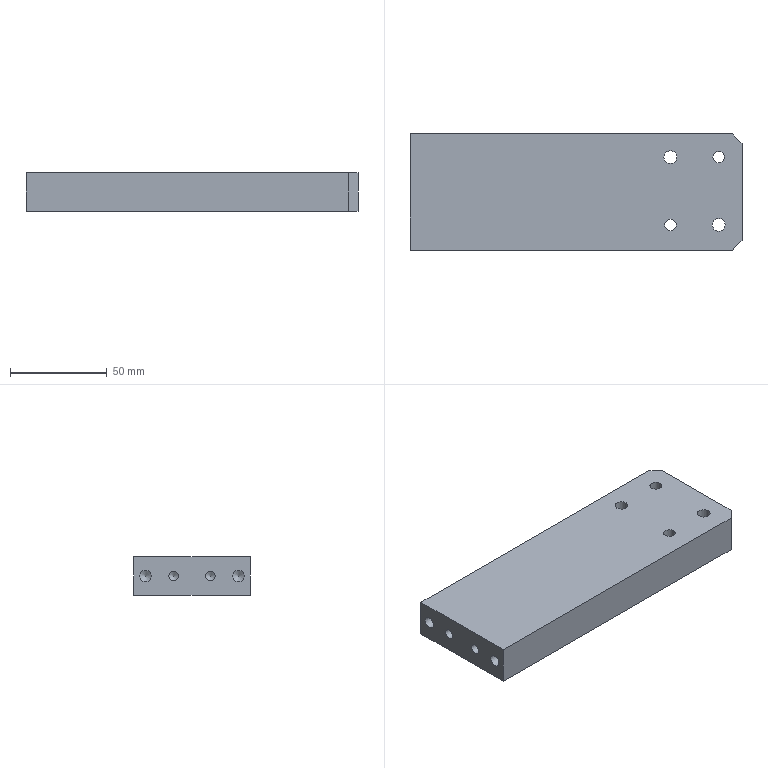Part | NX | features BREP 1 | 1 solid | 24 faces | box 171.5 x 60 x 20 mm | volume 200701 mm3 | plane 10 | cylinder 10 | cone 4 | commonest cylinder face diameters 6 x4 5 x2 6.6 x2 11 x2
STEP:
#1=CARTESIAN_POINT('',(-85.75,-30.,20.));
#2=VERTEX_POINT('',#1);
#3=CARTESIAN_POINT('',(80.75,-30.,20.));
#4=VERTEX_POINT('',#3);
#5=CARTESIAN_POINT('',(0.,-30.,20.));
#6=DIRECTION('',(1.,0.,0.));
#7=VECTOR('',#6,1000.);
#8=LINE('',#5,#7);
#9=EDGE_CURVE('',#2,#4,#8,.T.);
#10=ORIENTED_EDGE('',*,*,#9,.T.);
#11=CARTESIAN_POINT('',(85.75,-25.,20.));
#12=VERTEX_POINT('',#11);
#13=CARTESIAN_POINT('',(80.75,-30.,20.));
#14=DIRECTION('',(0.7071,0.7071,0.));
#15=VECTOR('',#14,1000.);
#16=LINE('',#13,#15);
#17=EDGE_CURVE('',#4,#12,#16,.T.);
#18=ORIENTED_EDGE('',*,*,#17,.T.);
#19=CARTESIAN_POINT('',(85.75,25.,20.));
#20=VERTEX_POINT('',#19);
#21=CARTESIAN_POINT('',(85.75,0.,20.));
#22=DIRECTION('',(0.,1.,0.));
#23=VECTOR('',#22,1000.);
#24=LINE('',#21,#23);
#25=EDGE_CURVE('',#12,#20,#24,.T.);
#26=ORIENTED_EDGE('',*,*,#25,.T.);
#27=CARTESIAN_POINT('',(80.75,30.,20.));
#28=VERTEX_POINT('',#27);
#29=CARTESIAN_POINT('',(85.75,25.,20.));
#30=DIRECTION('',(-0.7071,0.7071,0.));
#31=VECTOR('',#30,1000.);
#32=LINE('',#29,#31);
#33=EDGE_CURVE('',#20,#28,#32,.T.);
#34=ORIENTED_EDGE('',*,*,#33,.T.);
#35=CARTESIAN_POINT('',(-85.75,30.,20.));
#36=VERTEX_POINT('',#35);
#37=CARTESIAN_POINT('',(0.,30.,20.));
#38=DIRECTION('',(-1.,0.,0.));
#39=VECTOR('',#38,1000.);
#40=LINE('',#37,#39);
#41=EDGE_CURVE('',#28,#36,#40,.T.);
#42=ORIENTED_EDGE('',*,*,#41,.T.);
#43=CARTESIAN_POINT('',(-85.75,0.,20.));
#44=DIRECTION('',(0.,-1.,0.));
#45=VECTOR('',#44,1000.);
#46=LINE('',#43,#45);
#47=EDGE_CURVE('',#36,#2,#46,.T.);
#48=ORIENTED_EDGE('',*,*,#47,.T.);
#49=EDGE_LOOP('',(#10,#18,#26,#34,#42,#48));
#50=FACE_BOUND('',#49,.T.);
#51=CARTESIAN_POINT('',(51.75,-17.,20.));
#52=VERTEX_POINT('',#51);
#53=CARTESIAN_POINT('',(48.75,-17.,20.));
#54=DIRECTION('',(0.,0.,-1.));
#55=DIRECTION('',(1.,0.,0.));
#56=AXIS2_PLACEMENT_3D('',#53,#54,#55);
#57=CIRCLE('',#56,3.);
#58=EDGE_CURVE('',#52,#52,#57,.T.);
#59=ORIENTED_EDGE('',*,*,#58,.T.);
#60=EDGE_LOOP('',(#59));
#61=FACE_BOUND('',#60,.T.);
#62=CARTESIAN_POINT('',(76.75,18.,20.));
#63=VERTEX_POINT('',#62);
#64=CARTESIAN_POINT('',(73.75,18.,20.));
#65=DIRECTION('',(0.,0.,-1.));
#66=DIRECTION('',(1.,0.,0.));
#67=AXIS2_PLACEMENT_3D('',#64,#65,#66);
#68=CIRCLE('',#67,3.);
#69=EDGE_CURVE('',#63,#63,#68,.T.);
#70=ORIENTED_EDGE('',*,*,#69,.T.);
#71=EDGE_LOOP('',(#70));
#72=FACE_BOUND('',#71,.T.);
#73=CARTESIAN_POINT('',(45.45,18.,20.));
#74=VERTEX_POINT('',#73);
#75=CARTESIAN_POINT('',(48.75,18.,20.));
#76=DIRECTION('',(0.,0.,-1.));
#77=DIRECTION('',(-1.,0.,0.));
#78=AXIS2_PLACEMENT_3D('',#75,#76,#77);
#79=CIRCLE('',#78,3.3);
#80=EDGE_CURVE('',#74,#74,#79,.T.);
#81=ORIENTED_EDGE('',*,*,#80,.T.);
#82=EDGE_LOOP('',(#81));
#83=FACE_BOUND('',#82,.T.);
#84=CARTESIAN_POINT('',(70.45,-17.,20.));
#85=VERTEX_POINT('',#84);
#86=CARTESIAN_POINT('',(73.75,-17.,20.));
#87=DIRECTION('',(0.,0.,-1.));
#88=DIRECTION('',(-1.,0.,0.));
#89=AXIS2_PLACEMENT_3D('',#86,#87,#88);
#90=CIRCLE('',#89,3.3);
#91=EDGE_CURVE('',#85,#85,#90,.T.);
#92=ORIENTED_EDGE('',*,*,#91,.T.);
#93=EDGE_LOOP('',(#92));
#94=FACE_BOUND('',#93,.T.);
#95=CARTESIAN_POINT('',(0.,0.,20.));
#96=DIRECTION('',(0.,0.,1.));
#97=DIRECTION('',(-1.,0.,0.));
#98=AXIS2_PLACEMENT_3D('',#95,#96,#97);
#99=PLANE('',#98);
#100=ADVANCED_FACE('',(#50,#61,#72,#83,#94),#99,.T.);
#101=CARTESIAN_POINT('',(80.75,-30.,0.));
#102=VERTEX_POINT('',#101);
#103=CARTESIAN_POINT('',(80.75,-30.,20.));
#104=DIRECTION('',(0.,0.,1.));
#105=VECTOR('',#104,1000.);
#106=LINE('',#103,#105);
#107=EDGE_CURVE('',#102,#4,#106,.T.);
#108=ORIENTED_EDGE('',*,*,#107,.F.);
#109=CARTESIAN_POINT('',(85.75,-25.,0.));
#110=VERTEX_POINT('',#109);
#111=CARTESIAN_POINT('',(85.75,-25.,0.));
#112=DIRECTION('',(-0.7071,-0.7071,0.));
#113=VECTOR('',#112,1000.);
#114=LINE('',#111,#113);
#115=EDGE_CURVE('',#110,#102,#114,.T.);
#116=ORIENTED_EDGE('',*,*,#115,.F.);
#117=CARTESIAN_POINT('',(85.75,-25.,20.));
#118=DIRECTION('',(0.,0.,-1.));
#119=VECTOR('',#118,1000.);
#120=LINE('',#117,#119);
#121=EDGE_CURVE('',#12,#110,#120,.T.);
#122=ORIENTED_EDGE('',*,*,#121,.F.);
#123=ORIENTED_EDGE('',*,*,#17,.F.);
#124=EDGE_LOOP('',(#108,#116,#122,#123));
#125=FACE_BOUND('',#124,.T.);
#126=CARTESIAN_POINT('',(85.75,-25.,20.));
#127=DIRECTION('',(-0.7071,0.7071,0.));
#128=DIRECTION('',(0.7071,0.7071,0.));
#129=AXIS2_PLACEMENT_3D('',#126,#127,#128);
#130=PLANE('',#129);
#131=ADVANCED_FACE('',(#125),#130,.F.);
#132=ORIENTED_EDGE('',*,*,#107,.T.);
#133=ORIENTED_EDGE('',*,*,#9,.F.);
#134=CARTESIAN_POINT('',(-85.75,-30.,0.));
#135=VERTEX_POINT('',#134);
#136=CARTESIAN_POINT('',(-85.75,-30.,20.));
#137=DIRECTION('',(0.,0.,1.));
#138=VECTOR('',#137,1000.);
#139=LINE('',#136,#138);
#140=EDGE_CURVE('',#135,#2,#139,.T.);
#141=ORIENTED_EDGE('',*,*,#140,.F.);
#142=CARTESIAN_POINT('',(-85.75,-30.,0.));
#143=DIRECTION('',(-1.,0.,0.));
#144=VECTOR('',#143,1000.);
#145=LINE('',#142,#144);
#146=EDGE_CURVE('',#102,#135,#145,.T.);
#147=ORIENTED_EDGE('',*,*,#146,.F.);
#148=EDGE_LOOP('',(#132,#133,#141,#147));
#149=FACE_BOUND('',#148,.T.);
#150=CARTESIAN_POINT('',(-85.75,-30.,20.));
#151=DIRECTION('',(0.,1.,0.));
#152=DIRECTION('',(0.,0.,-1.));
#153=AXIS2_PLACEMENT_3D('',#150,#151,#152);
#154=PLANE('',#153);
#155=ADVANCED_FACE('',(#149),#154,.F.);
#156=ORIENTED_EDGE('',*,*,#140,.T.);
#157=ORIENTED_EDGE('',*,*,#47,.F.);
#158=CARTESIAN_POINT('',(-85.75,30.,0.));
#159=VERTEX_POINT('',#158);
#160=CARTESIAN_POINT('',(-85.75,30.,20.));
#161=DIRECTION('',(0.,0.,1.));
#162=VECTOR('',#161,1000.);
#163=LINE('',#160,#162);
#164=EDGE_CURVE('',#159,#36,#163,.T.);
#165=ORIENTED_EDGE('',*,*,#164,.F.);
#166=CARTESIAN_POINT('',(-85.75,30.,0.));
#167=DIRECTION('',(0.,1.,0.));
#168=VECTOR('',#167,1000.);
#169=LINE('',#166,#168);
#170=EDGE_CURVE('',#135,#159,#169,.T.);
#171=ORIENTED_EDGE('',*,*,#170,.F.);
#172=EDGE_LOOP('',(#156,#157,#165,#171));
#173=FACE_BOUND('',#172,.T.);
#174=CARTESIAN_POINT('',(-85.75,-24.,13.));
#175=VERTEX_POINT('',#174);
#176=CARTESIAN_POINT('',(-85.75,-24.,10.));
#177=DIRECTION('',(-1.,0.,0.));
#178=DIRECTION('',(0.,0.,1.));
#179=AXIS2_PLACEMENT_3D('',#176,#177,#178);
#180=CIRCLE('',#179,3.);
#181=EDGE_CURVE('',#175,#175,#180,.T.);
#182=ORIENTED_EDGE('',*,*,#181,.F.);
#183=EDGE_LOOP('',(#182));
#184=FACE_BOUND('',#183,.T.);
#185=CARTESIAN_POINT('',(-85.75,24.,13.));
#186=VERTEX_POINT('',#185);
#187=CARTESIAN_POINT('',(-85.75,24.,10.));
#188=DIRECTION('',(-1.,0.,0.));
#189=DIRECTION('',(0.,0.,1.));
#190=AXIS2_PLACEMENT_3D('',#187,#188,#189);
#191=CIRCLE('',#190,3.);
#192=EDGE_CURVE('',#186,#186,#191,.T.);
#193=ORIENTED_EDGE('',*,*,#192,.F.);
#194=EDGE_LOOP('',(#193));
#195=FACE_BOUND('',#194,.T.);
#196=CARTESIAN_POINT('',(-85.75,9.5,12.5));
#197=VERTEX_POINT('',#196);
#198=CARTESIAN_POINT('',(-85.75,9.5,10.));
#199=DIRECTION('',(-1.,0.,0.));
#200=DIRECTION('',(0.,0.,1.));
#201=AXIS2_PLACEMENT_3D('',#198,#199,#200);
#202=CIRCLE('',#201,2.5);
#203=EDGE_CURVE('',#197,#197,#202,.T.);
#204=ORIENTED_EDGE('',*,*,#203,.F.);
#205=EDGE_LOOP('',(#204));
#206=FACE_BOUND('',#205,.T.);
#207=CARTESIAN_POINT('',(-85.75,-9.5,12.5));
#208=VERTEX_POINT('',#207);
#209=CARTESIAN_POINT('',(-85.75,-9.5,10.));
#210=DIRECTION('',(-1.,0.,0.));
#211=DIRECTION('',(0.,0.,1.));
#212=AXIS2_PLACEMENT_3D('',#209,#210,#211);
#213=CIRCLE('',#212,2.5);
#214=EDGE_CURVE('',#208,#208,#213,.T.);
#215=ORIENTED_EDGE('',*,*,#214,.F.);
#216=EDGE_LOOP('',(#215));
#217=FACE_BOUND('',#216,.T.);
#218=CARTESIAN_POINT('',(-85.75,30.,20.));
#219=DIRECTION('',(1.,0.,0.));
#220=DIRECTION('',(0.,-1.,0.));
#221=AXIS2_PLACEMENT_3D('',#218,#219,#220);
#222=PLANE('',#221);
#223=ADVANCED_FACE('',(#173,#184,#195,#206,#217),#222,.F.);
#224=CARTESIAN_POINT('',(80.75,30.,0.));
#225=VERTEX_POINT('',#224);
#226=CARTESIAN_POINT('',(80.75,30.,20.));
#227=DIRECTION('',(0.,0.,1.));
#228=VECTOR('',#227,1000.);
#229=LINE('',#226,#228);
#230=EDGE_CURVE('',#225,#28,#229,.T.);
#231=ORIENTED_EDGE('',*,*,#230,.F.);
#232=CARTESIAN_POINT('',(-85.75,30.,0.));
#233=DIRECTION('',(1.,0.,0.));
#234=VECTOR('',#233,1000.);
#235=LINE('',#232,#234);
#236=EDGE_CURVE('',#159,#225,#235,.T.);
#237=ORIENTED_EDGE('',*,*,#236,.F.);
#238=ORIENTED_EDGE('',*,*,#164,.T.);
#239=ORIENTED_EDGE('',*,*,#41,.F.);
#240=EDGE_LOOP('',(#231,#237,#238,#239));
#241=FACE_BOUND('',#240,.T.);
#242=CARTESIAN_POINT('',(-85.75,30.,20.));
#243=DIRECTION('',(0.,-1.,0.));
#244=DIRECTION('',(0.,0.,1.));
#245=AXIS2_PLACEMENT_3D('',#242,#243,#244);
#246=PLANE('',#245);
#247=ADVANCED_FACE('',(#241),#246,.F.);
#248=CARTESIAN_POINT('',(85.75,25.,0.));
#249=VERTEX_POINT('',#248);
#250=CARTESIAN_POINT('',(85.75,25.,20.));
#251=DIRECTION('',(0.,0.,1.));
#252=VECTOR('',#251,1000.);
#253=LINE('',#250,#252);
#254=EDGE_CURVE('',#249,#20,#253,.T.);
#255=ORIENTED_EDGE('',*,*,#254,.F.);
#256=CARTESIAN_POINT('',(80.75,30.,0.));
#257=DIRECTION('',(0.7071,-0.7071,0.));
#258=VECTOR('',#257,1000.);
#259=LINE('',#256,#258);
#260=EDGE_CURVE('',#225,#249,#259,.T.);
#261=ORIENTED_EDGE('',*,*,#260,.F.);
#262=ORIENTED_EDGE('',*,*,#230,.T.);
#263=ORIENTED_EDGE('',*,*,#33,.F.);
#264=EDGE_LOOP('',(#255,#261,#262,#263));
#265=FACE_BOUND('',#264,.T.);
#266=CARTESIAN_POINT('',(80.75,30.,20.));
#267=DIRECTION('',(-0.7071,-0.7071,0.));
#268=DIRECTION('',(-0.7071,0.7071,0.));
#269=AXIS2_PLACEMENT_3D('',#266,#267,#268);
#270=PLANE('',#269);
#271=ADVANCED_FACE('',(#265),#270,.F.);
#272=ORIENTED_EDGE('',*,*,#254,.T.);
#273=ORIENTED_EDGE('',*,*,#25,.F.);
#274=ORIENTED_EDGE('',*,*,#121,.T.);
#275=CARTESIAN_POINT('',(85.75,30.,0.));
#276=DIRECTION('',(0.,-1.,0.));
#277=VECTOR('',#276,1000.);
#278=LINE('',#275,#277);
#279=EDGE_CURVE('',#249,#110,#278,.T.);
#280=ORIENTED_EDGE('',*,*,#279,.F.);
#281=EDGE_LOOP('',(#272,#273,#274,#280));
#282=FACE_BOUND('',#281,.T.);
#283=CARTESIAN_POINT('',(85.75,30.,20.));
#284=DIRECTION('',(-1.,0.,0.));
#285=DIRECTION('',(0.,1.,0.));
#286=AXIS2_PLACEMENT_3D('',#283,#284,#285);
#287=PLANE('',#286);
#288=ADVANCED_FACE('',(#282),#287,.F.);
#289=ORIENTED_EDGE('',*,*,#58,.F.);
#290=EDGE_LOOP('',(#289));
#291=FACE_BOUND('',#290,.T.);
#292=CARTESIAN_POINT('',(51.75,-17.,0.));
#293=VERTEX_POINT('',#292);
#294=CARTESIAN_POINT('',(48.75,-17.,0.));
#295=DIRECTION('',(0.,0.,1.));
#296=DIRECTION('',(1.,0.,0.));
#297=AXIS2_PLACEMENT_3D('',#294,#295,#296);
#298=CIRCLE('',#297,3.);
#299=EDGE_CURVE('',#293,#293,#298,.T.);
#300=ORIENTED_EDGE('',*,*,#299,.F.);
#301=EDGE_LOOP('',(#300));
#302=FACE_BOUND('',#301,.T.);
#303=CARTESIAN_POINT('',(48.75,-17.,20.));
#304=DIRECTION('',(0.,0.,1.));
#305=DIRECTION('',(-1.,0.,0.));
#306=AXIS2_PLACEMENT_3D('',#303,#304,#305);
#307=CYLINDRICAL_SURFACE('',#306,3.);
#308=ADVANCED_FACE('',(#291,#302),#307,.F.);
#309=ORIENTED_EDGE('',*,*,#69,.F.);
#310=EDGE_LOOP('',(#309));
#311=FACE_BOUND('',#310,.T.);
#312=CARTESIAN_POINT('',(76.75,18.,0.));
#313=VERTEX_POINT('',#312);
#314=CARTESIAN_POINT('',(73.75,18.,0.));
#315=DIRECTION('',(0.,0.,1.));
#316=DIRECTION('',(1.,0.,0.));
#317=AXIS2_PLACEMENT_3D('',#314,#315,#316);
#318=CIRCLE('',#317,3.);
#319=EDGE_CURVE('',#313,#313,#318,.T.);
#320=ORIENTED_EDGE('',*,*,#319,.F.);
#321=EDGE_LOOP('',(#320));
#322=FACE_BOUND('',#321,.T.);
#323=CARTESIAN_POINT('',(73.75,18.,20.));
#324=DIRECTION('',(0.,0.,1.));
#325=DIRECTION('',(-1.,0.,0.));
#326=AXIS2_PLACEMENT_3D('',#323,#324,#325);
#327=CYLINDRICAL_SURFACE('',#326,3.);
#328=ADVANCED_FACE('',(#311,#322),#327,.F.);
#329=CARTESIAN_POINT('',(45.45,18.,6.4));
#330=VERTEX_POINT('',#329);
#331=CARTESIAN_POINT('',(48.75,18.,6.4));
#332=DIRECTION('',(0.,0.,1.));
#333=DIRECTION('',(-1.,0.,0.));
#334=AXIS2_PLACEMENT_3D('',#331,#332,#333);
#335=CIRCLE('',#334,3.3);
#336=EDGE_CURVE('',#330,#330,#335,.T.);
#337=ORIENTED_EDGE('',*,*,#336,.F.);
#338=EDGE_LOOP('',(#337));
#339=FACE_BOUND('',#338,.T.);
#340=ORIENTED_EDGE('',*,*,#80,.F.);
#341=EDGE_LOOP('',(#340));
#342=FACE_BOUND('',#341,.T.);
#343=CARTESIAN_POINT('',(48.75,18.,0.));
#344=DIRECTION('',(0.,0.,-1.));
#345=DIRECTION('',(1.,0.,0.));
#346=AXIS2_PLACEMENT_3D('',#343,#344,#345);
#347=CYLINDRICAL_SURFACE('',#346,3.3);
#348=ADVANCED_FACE('',(#339,#342),#347,.F.);
#349=CARTESIAN_POINT('',(70.45,-17.,6.4));
#350=VERTEX_POINT('',#349);
#351=CARTESIAN_POINT('',(73.75,-17.,6.4));
#352=DIRECTION('',(0.,0.,1.));
#353=DIRECTION('',(-1.,0.,0.));
#354=AXIS2_PLACEMENT_3D('',#351,#352,#353);
#355=CIRCLE('',#354,3.3);
#356=EDGE_CURVE('',#350,#350,#355,.T.);
#357=ORIENTED_EDGE('',*,*,#356,.F.);
#358=EDGE_LOOP('',(#357));
#359=FACE_BOUND('',#358,.T.);
#360=ORIENTED_EDGE('',*,*,#91,.F.);
#361=EDGE_LOOP('',(#360));
#362=FACE_BOUND('',#361,.T.);
#363=CARTESIAN_POINT('',(73.75,-17.,0.));
#364=DIRECTION('',(0.,0.,-1.));
#365=DIRECTION('',(1.,0.,0.));
#366=AXIS2_PLACEMENT_3D('',#363,#364,#365);
#367=CYLINDRICAL_SURFACE('',#366,3.3);
#368=ADVANCED_FACE('',(#359,#362),#367,.F.);
#369=ORIENTED_EDGE('',*,*,#260,.T.);
#370=ORIENTED_EDGE('',*,*,#279,.T.);
#371=ORIENTED_EDGE('',*,*,#115,.T.);
#372=ORIENTED_EDGE('',*,*,#146,.T.);
#373=ORIENTED_EDGE('',*,*,#170,.T.);
#374=ORIENTED_EDGE('',*,*,#236,.T.);
#375=EDGE_LOOP('',(#369,#370,#371,#372,#373,#374));
#376=FACE_BOUND('',#375,.T.);
#377=ORIENTED_EDGE('',*,*,#299,.T.);
#378=EDGE_LOOP('',(#377));
#379=FACE_BOUND('',#378,.T.);
#380=ORIENTED_EDGE('',*,*,#319,.T.);
#381=EDGE_LOOP('',(#380));
#382=FACE_BOUND('',#381,.T.);
#383=CARTESIAN_POINT('',(43.25,18.,0.));
#384=VERTEX_POINT('',#383);
#385=CARTESIAN_POINT('',(48.75,18.,0.));
#386=DIRECTION('',(0.,0.,-1.));
#387=DIRECTION('',(-1.,0.,0.));
#388=AXIS2_PLACEMENT_3D('',#385,#386,#387);
#389=CIRCLE('',#388,5.5);
#390=EDGE_CURVE('',#384,#384,#389,.T.);
#391=ORIENTED_EDGE('',*,*,#390,.F.);
#392=EDGE_LOOP('',(#391));
#393=FACE_BOUND('',#392,.T.);
#394=CARTESIAN_POINT('',(68.25,-17.,0.));
#395=VERTEX_POINT('',#394);
#396=CARTESIAN_POINT('',(73.75,-17.,0.));
#397=DIRECTION('',(0.,0.,-1.));
#398=DIRECTION('',(-1.,0.,0.));
#399=AXIS2_PLACEMENT_3D('',#396,#397,#398);
#400=CIRCLE('',#399,5.5);
#401=EDGE_CURVE('',#395,#395,#400,.T.);
#402=ORIENTED_EDGE('',*,*,#401,.F.);
#403=EDGE_LOOP('',(#402));
#404=FACE_BOUND('',#403,.T.);
#405=CARTESIAN_POINT('',(0.,0.,0.));
#406=DIRECTION('',(0.,0.,1.));
#407=DIRECTION('',(-1.,0.,0.));
#408=AXIS2_PLACEMENT_3D('',#405,#406,#407);
#409=PLANE('',#408);
#410=ADVANCED_FACE('',(#376,#379,#382,#393,#404),#409,.F.);
#411=CARTESIAN_POINT('',(-73.75,-24.,13.));
#412=VERTEX_POINT('',#411);
#413=CARTESIAN_POINT('',(-73.75,-24.,10.));
#414=DIRECTION('',(-1.,0.,0.));
#415=DIRECTION('',(0.,0.,1.));
#416=AXIS2_PLACEMENT_3D('',#413,#414,#415);
#417=CIRCLE('',#416,3.);
#418=EDGE_CURVE('',#412,#412,#417,.T.);
#419=ORIENTED_EDGE('',*,*,#418,.F.);
#420=EDGE_LOOP('',(#419));
#421=FACE_BOUND('',#420,.T.);
#422=ORIENTED_EDGE('',*,*,#181,.T.);
#423=EDGE_LOOP('',(#422));
#424=FACE_BOUND('',#423,.T.);
#425=CARTESIAN_POINT('',(-85.75,-24.,10.));
#426=DIRECTION('',(-1.,0.,0.));
#427=DIRECTION('',(0.,0.,-1.));
#428=AXIS2_PLACEMENT_3D('',#425,#426,#427);
#429=CYLINDRICAL_SURFACE('',#428,3.);
#430=ADVANCED_FACE('',(#421,#424),#429,.F.);
#431=CARTESIAN_POINT('',(-73.75,24.,13.));
#432=VERTEX_POINT('',#431);
#433=CARTESIAN_POINT('',(-73.75,24.,10.));
#434=DIRECTION('',(-1.,0.,0.));
#435=DIRECTION('',(0.,0.,1.));
#436=AXIS2_PLACEMENT_3D('',#433,#434,#435);
#437=CIRCLE('',#436,3.);
#438=EDGE_CURVE('',#432,#432,#437,.T.);
#439=ORIENTED_EDGE('',*,*,#438,.F.);
#440=EDGE_LOOP('',(#439));
#441=FACE_BOUND('',#440,.T.);
#442=ORIENTED_EDGE('',*,*,#192,.T.);
#443=EDGE_LOOP('',(#442));
#444=FACE_BOUND('',#443,.T.);
#445=CARTESIAN_POINT('',(-85.75,24.,10.));
#446=DIRECTION('',(-1.,0.,0.));
#447=DIRECTION('',(0.,0.,-1.));
#448=AXIS2_PLACEMENT_3D('',#445,#446,#447);
#449=CYLINDRICAL_SURFACE('',#448,3.);
#450=ADVANCED_FACE('',(#441,#444),#449,.F.);
#451=CARTESIAN_POINT('',(-70.75,9.5,12.5));
#452=VERTEX_POINT('',#451);
#453=CARTESIAN_POINT('',(-70.75,9.5,10.));
#454=DIRECTION('',(-1.,0.,0.));
#455=DIRECTION('',(0.,0.,1.));
#456=AXIS2_PLACEMENT_3D('',#453,#454,#455);
#457=CIRCLE('',#456,2.5);
#458=EDGE_CURVE('',#452,#452,#457,.T.);
#459=ORIENTED_EDGE('',*,*,#458,.F.);
#460=EDGE_LOOP('',(#459));
#461=FACE_BOUND('',#460,.T.);
#462=ORIENTED_EDGE('',*,*,#203,.T.);
#463=EDGE_LOOP('',(#462));
#464=FACE_BOUND('',#463,.T.);
#465=CARTESIAN_POINT('',(-85.75,9.5,10.));
#466=DIRECTION('',(-1.,0.,0.));
#467=DIRECTION('',(0.,0.,-1.));
#468=AXIS2_PLACEMENT_3D('',#465,#466,#467);
#469=CYLINDRICAL_SURFACE('',#468,2.5);
#470=ADVANCED_FACE('',(#461,#464),#469,.F.);
#471=CARTESIAN_POINT('',(-70.75,-9.5,12.5));
#472=VERTEX_POINT('',#471);
#473=CARTESIAN_POINT('',(-70.75,-9.5,10.));
#474=DIRECTION('',(-1.,0.,0.));
#475=DIRECTION('',(0.,0.,1.));
#476=AXIS2_PLACEMENT_3D('',#473,#474,#475);
#477=CIRCLE('',#476,2.5);
#478=EDGE_CURVE('',#472,#472,#477,.T.);
#479=ORIENTED_EDGE('',*,*,#478,.F.);
#480=EDGE_LOOP('',(#479));
#481=FACE_BOUND('',#480,.T.);
#482=ORIENTED_EDGE('',*,*,#214,.T.);
#483=EDGE_LOOP('',(#482));
#484=FACE_BOUND('',#483,.T.);
#485=CARTESIAN_POINT('',(-85.75,-9.5,10.));
#486=DIRECTION('',(-1.,0.,0.));
#487=DIRECTION('',(0.,0.,-1.));
#488=AXIS2_PLACEMENT_3D('',#485,#486,#487);
#489=CYLINDRICAL_SURFACE('',#488,2.5);
#490=ADVANCED_FACE('',(#481,#484),#489,.F.);
#491=CARTESIAN_POINT('',(43.25,18.,6.4));
#492=VERTEX_POINT('',#491);
#493=CARTESIAN_POINT('',(48.75,18.,6.4));
#494=DIRECTION('',(0.,0.,1.));
#495=DIRECTION('',(-1.,0.,0.));
#496=AXIS2_PLACEMENT_3D('',#493,#494,#495);
#497=CIRCLE('',#496,5.5);
#498=EDGE_CURVE('',#492,#492,#497,.T.);
#499=ORIENTED_EDGE('',*,*,#498,.F.);
#500=EDGE_LOOP('',(#499));
#501=FACE_BOUND('',#500,.T.);
#502=ORIENTED_EDGE('',*,*,#336,.T.);
#503=EDGE_LOOP('',(#502));
#504=FACE_BOUND('',#503,.T.);
#505=CARTESIAN_POINT('',(52.05,18.,6.4));
#506=DIRECTION('',(0.,0.,1.));
#507=DIRECTION('',(-1.,0.,0.));
#508=AXIS2_PLACEMENT_3D('',#505,#506,#507);
#509=PLANE('',#508);
#510=ADVANCED_FACE('',(#501,#504),#509,.F.);
#511=CARTESIAN_POINT('',(68.25,-17.,6.4));
#512=VERTEX_POINT('',#511);
#513=CARTESIAN_POINT('',(73.75,-17.,6.4));
#514=DIRECTION('',(0.,0.,1.));
#515=DIRECTION('',(-1.,0.,0.));
#516=AXIS2_PLACEMENT_3D('',#513,#514,#515);
#517=CIRCLE('',#516,5.5);
#518=EDGE_CURVE('',#512,#512,#517,.T.);
#519=ORIENTED_EDGE('',*,*,#518,.F.);
#520=EDGE_LOOP('',(#519));
#521=FACE_BOUND('',#520,.T.);
#522=ORIENTED_EDGE('',*,*,#356,.T.);
#523=EDGE_LOOP('',(#522));
#524=FACE_BOUND('',#523,.T.);
#525=CARTESIAN_POINT('',(77.05,-17.,6.4));
#526=DIRECTION('',(0.,0.,1.));
#527=DIRECTION('',(-1.,0.,0.));
#528=AXIS2_PLACEMENT_3D('',#525,#526,#527);
#529=PLANE('',#528);
#530=ADVANCED_FACE('',(#521,#524),#529,.F.);
#531=ORIENTED_EDGE('',*,*,#498,.T.);
#532=EDGE_LOOP('',(#531));
#533=FACE_BOUND('',#532,.T.);
#534=ORIENTED_EDGE('',*,*,#390,.T.);
#535=EDGE_LOOP('',(#534));
#536=FACE_BOUND('',#535,.T.);
#537=CARTESIAN_POINT('',(48.75,18.,0.));
#538=DIRECTION('',(0.,0.,-1.));
#539=DIRECTION('',(1.,0.,0.));
#540=AXIS2_PLACEMENT_3D('',#537,#538,#539);
#541=CYLINDRICAL_SURFACE('',#540,5.5);
#542=ADVANCED_FACE('',(#533,#536),#541,.F.);
#543=ORIENTED_EDGE('',*,*,#518,.T.);
#544=EDGE_LOOP('',(#543));
#545=FACE_BOUND('',#544,.T.);
#546=ORIENTED_EDGE('',*,*,#401,.T.);
#547=EDGE_LOOP('',(#546));
#548=FACE_BOUND('',#547,.T.);
#549=CARTESIAN_POINT('',(73.75,-17.,0.));
#550=DIRECTION('',(0.,0.,-1.));
#551=DIRECTION('',(1.,0.,0.));
#552=AXIS2_PLACEMENT_3D('',#549,#550,#551);
#553=CYLINDRICAL_SURFACE('',#552,5.5);
#554=ADVANCED_FACE('',(#545,#548),#553,.F.);
#555=CARTESIAN_POINT('',(-71.947,-24.,10.));
#556=VERTEX_POINT('',#555);
#557=VERTEX_LOOP('',#556);
#558=FACE_BOUND('',#557,.T.);
#559=ORIENTED_EDGE('',*,*,#418,.T.);
#560=EDGE_LOOP('',(#559));
#561=FACE_BOUND('',#560,.T.);
#562=CARTESIAN_POINT('',(-73.75,-24.,10.));
#563=DIRECTION('',(-1.,0.,0.));
#564=DIRECTION('',(0.,0.,-1.));
#565=AXIS2_PLACEMENT_3D('',#562,#563,#564);
#566=CONICAL_SURFACE('',#565,3.,1.03);
#567=ADVANCED_FACE('',(#558,#561),#566,.F.);
#568=CARTESIAN_POINT('',(-71.947,24.,10.));
#569=VERTEX_POINT('',#568);
#570=VERTEX_LOOP('',#569);
#571=FACE_BOUND('',#570,.T.);
#572=ORIENTED_EDGE('',*,*,#438,.T.);
#573=EDGE_LOOP('',(#572));
#574=FACE_BOUND('',#573,.T.);
#575=CARTESIAN_POINT('',(-73.75,24.,10.));
#576=DIRECTION('',(-1.,0.,0.));
#577=DIRECTION('',(0.,0.,-1.));
#578=AXIS2_PLACEMENT_3D('',#575,#576,#577);
#579=CONICAL_SURFACE('',#578,3.,1.03);
#580=ADVANCED_FACE('',(#571,#574),#579,.F.);
#581=CARTESIAN_POINT('',(-69.248,9.5,10.));
#582=VERTEX_POINT('',#581);
#583=VERTEX_LOOP('',#582);
#584=FACE_BOUND('',#583,.T.);
#585=ORIENTED_EDGE('',*,*,#458,.T.);
#586=EDGE_LOOP('',(#585));
#587=FACE_BOUND('',#586,.T.);
#588=CARTESIAN_POINT('',(-70.75,9.5,10.));
#589=DIRECTION('',(-1.,0.,0.));
#590=DIRECTION('',(0.,0.,-1.));
#591=AXIS2_PLACEMENT_3D('',#588,#589,#590);
#592=CONICAL_SURFACE('',#591,2.5,1.03);
#593=ADVANCED_FACE('',(#584,#587),#592,.F.);
#594=CARTESIAN_POINT('',(-69.248,-9.5,10.));
#595=VERTEX_POINT('',#594);
#596=VERTEX_LOOP('',#595);
#597=FACE_BOUND('',#596,.T.);
#598=ORIENTED_EDGE('',*,*,#478,.T.);
#599=EDGE_LOOP('',(#598));
#600=FACE_BOUND('',#599,.T.);
#601=CARTESIAN_POINT('',(-70.75,-9.5,10.));
#602=DIRECTION('',(-1.,0.,0.));
#603=DIRECTION('',(0.,0.,-1.));
#604=AXIS2_PLACEMENT_3D('',#601,#602,#603);
#605=CONICAL_SURFACE('',#604,2.5,1.03);
#606=ADVANCED_FACE('',(#597,#600),#605,.F.);
#607=CLOSED_SHELL('',(#100,#131,#155,#223,#247,#271,#288,#308,#328,#348,#368,#410,#430,#450,#470,#490,#510,#530,#542,#554,#567,#580,#593,#606));
#608=MANIFOLD_SOLID_BREP('',#607);
#609=(LENGTH_UNIT()NAMED_UNIT(*)SI_UNIT(.MILLI.,.METRE.));
#610=UNCERTAINTY_MEASURE_WITH_UNIT(LENGTH_MEASURE(0.00001),#609,'','');
#611=(NAMED_UNIT(*)PLANE_ANGLE_UNIT()SI_UNIT($,.RADIAN.));
#612=(NAMED_UNIT(*)SI_UNIT($,.STERADIAN.)SOLID_ANGLE_UNIT());
#613=(GEOMETRIC_REPRESENTATION_CONTEXT(3)GLOBAL_UNCERTAINTY_ASSIGNED_CONTEXT((#610))GLOBAL_UNIT_ASSIGNED_CONTEXT((#609,#611,#612))REPRESENTATION_CONTEXT('',''));
#614=ADVANCED_BREP_SHAPE_REPRESENTATION('',(#608),#613);